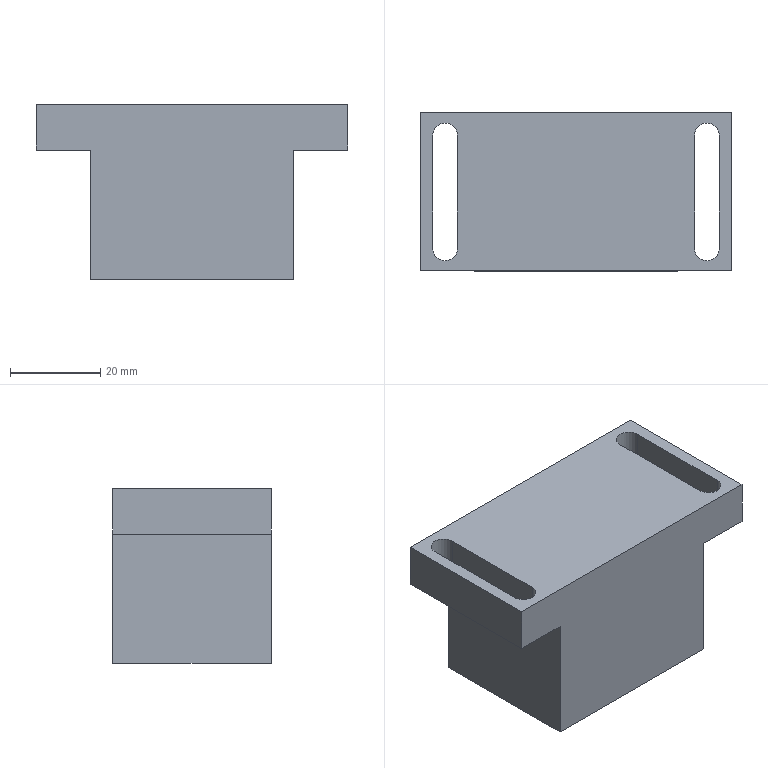Part | STEP file | 11-FG-S00711 | 1 solid | 34 faces | box 69 x 35 x 38.6 mm | volume 65613 mm3 | plane 14 | cylinder 12 | cone 8 | commonest cylinder face diameters 3.3 x8 5.5 x4
STEP:
#1=CARTESIAN_POINT('',(44.15,-7.,10.1));
#2=VERTEX_POINT('',#1);
#3=CARTESIAN_POINT('',(40.85,-7.,10.1));
#4=VERTEX_POINT('',#3);
#5=CARTESIAN_POINT('',(42.5,-7.,10.1));
#6=DIRECTION('',(0.,0.,-1.));
#7=DIRECTION('',(-1.,0.,0.));
#8=AXIS2_PLACEMENT_3D('',#5,#6,#7);
#9=CIRCLE('',#8,1.65);
#10=EDGE_CURVE('',#2,#4,#9,.T.);
#11=ORIENTED_EDGE('',*,*,#10,.F.);
#12=CARTESIAN_POINT('',(44.15,-7.,0.));
#13=VERTEX_POINT('',#12);
#14=CARTESIAN_POINT('',(44.15,-7.,0.));
#15=DIRECTION('',(0.,0.,-1.));
#16=VECTOR('',#15,1000.);
#17=LINE('',#14,#16);
#18=EDGE_CURVE('',#2,#13,#17,.T.);
#19=ORIENTED_EDGE('',*,*,#18,.T.);
#20=CARTESIAN_POINT('',(40.85,-7.,0.));
#21=VERTEX_POINT('',#20);
#22=CARTESIAN_POINT('',(42.5,-7.,0.));
#23=DIRECTION('',(0.,0.,-1.));
#24=DIRECTION('',(-1.,0.,0.));
#25=AXIS2_PLACEMENT_3D('',#22,#23,#24);
#26=CIRCLE('',#25,1.65);
#27=EDGE_CURVE('',#13,#21,#26,.T.);
#28=ORIENTED_EDGE('',*,*,#27,.T.);
#29=CARTESIAN_POINT('',(40.85,-7.,0.));
#30=DIRECTION('',(0.,0.,-1.));
#31=VECTOR('',#30,1000.);
#32=LINE('',#29,#31);
#33=EDGE_CURVE('',#4,#21,#32,.T.);
#34=ORIENTED_EDGE('',*,*,#33,.F.);
#35=EDGE_LOOP('',(#11,#19,#28,#34));
#36=FACE_OUTER_BOUND('',#35,.T.);
#37=CARTESIAN_POINT('',(42.5,-7.,0.));
#38=DIRECTION('',(0.,0.,-1.));
#39=DIRECTION('',(-1.,0.,0.));
#40=AXIS2_PLACEMENT_3D('',#37,#38,#39);
#41=CYLINDRICAL_SURFACE('',#40,1.65);
#42=ADVANCED_FACE('',(#36),#41,.F.);
#43=CARTESIAN_POINT('',(42.5,-7.,11.091));
#44=VERTEX_POINT('',#43);
#45=CARTESIAN_POINT('',(40.85,-7.,10.1));
#46=DIRECTION('',(-0.8572,0.,-0.515));
#47=VECTOR('',#46,1000.);
#48=LINE('',#45,#47);
#49=EDGE_CURVE('',#44,#4,#48,.T.);
#50=ORIENTED_EDGE('',*,*,#49,.F.);
#51=CARTESIAN_POINT('',(44.15,-7.,10.1));
#52=DIRECTION('',(0.8572,0.,-0.515));
#53=VECTOR('',#52,1000.);
#54=LINE('',#51,#53);
#55=EDGE_CURVE('',#44,#2,#54,.T.);
#56=ORIENTED_EDGE('',*,*,#55,.T.);
#57=ORIENTED_EDGE('',*,*,#10,.T.);
#58=EDGE_LOOP('',(#50,#56,#57));
#59=FACE_OUTER_BOUND('',#58,.T.);
#60=CARTESIAN_POINT('',(42.5,-7.,10.1));
#61=DIRECTION('',(0.,0.,-1.));
#62=DIRECTION('',(-1.,0.,0.));
#63=AXIS2_PLACEMENT_3D('',#60,#61,#62);
#64=CONICAL_SURFACE('',#63,1.65,1.03);
#65=ADVANCED_FACE('',(#59),#64,.F.);
#66=CARTESIAN_POINT('',(44.15,-28.,10.1));
#67=VERTEX_POINT('',#66);
#68=CARTESIAN_POINT('',(40.85,-28.,10.1));
#69=VERTEX_POINT('',#68);
#70=CARTESIAN_POINT('',(42.5,-28.,10.1));
#71=DIRECTION('',(0.,0.,-1.));
#72=DIRECTION('',(-1.,0.,0.));
#73=AXIS2_PLACEMENT_3D('',#70,#71,#72);
#74=CIRCLE('',#73,1.65);
#75=EDGE_CURVE('',#67,#69,#74,.T.);
#76=ORIENTED_EDGE('',*,*,#75,.F.);
#77=CARTESIAN_POINT('',(44.15,-28.,0.));
#78=VERTEX_POINT('',#77);
#79=CARTESIAN_POINT('',(44.15,-28.,0.));
#80=DIRECTION('',(0.,0.,-1.));
#81=VECTOR('',#80,1000.);
#82=LINE('',#79,#81);
#83=EDGE_CURVE('',#67,#78,#82,.T.);
#84=ORIENTED_EDGE('',*,*,#83,.T.);
#85=CARTESIAN_POINT('',(40.85,-28.,0.));
#86=VERTEX_POINT('',#85);
#87=CARTESIAN_POINT('',(42.5,-28.,0.));
#88=DIRECTION('',(0.,0.,-1.));
#89=DIRECTION('',(-1.,0.,0.));
#90=AXIS2_PLACEMENT_3D('',#87,#88,#89);
#91=CIRCLE('',#90,1.65);
#92=EDGE_CURVE('',#78,#86,#91,.T.);
#93=ORIENTED_EDGE('',*,*,#92,.T.);
#94=CARTESIAN_POINT('',(40.85,-28.,0.));
#95=DIRECTION('',(0.,0.,-1.));
#96=VECTOR('',#95,1000.);
#97=LINE('',#94,#96);
#98=EDGE_CURVE('',#69,#86,#97,.T.);
#99=ORIENTED_EDGE('',*,*,#98,.F.);
#100=EDGE_LOOP('',(#76,#84,#93,#99));
#101=FACE_OUTER_BOUND('',#100,.T.);
#102=CARTESIAN_POINT('',(42.5,-28.,0.));
#103=DIRECTION('',(0.,0.,-1.));
#104=DIRECTION('',(-1.,0.,0.));
#105=AXIS2_PLACEMENT_3D('',#102,#103,#104);
#106=CYLINDRICAL_SURFACE('',#105,1.65);
#107=ADVANCED_FACE('',(#101),#106,.F.);
#108=CARTESIAN_POINT('',(42.5,-28.,11.091));
#109=VERTEX_POINT('',#108);
#110=CARTESIAN_POINT('',(40.85,-28.,10.1));
#111=DIRECTION('',(-0.8572,0.,-0.515));
#112=VECTOR('',#111,1000.);
#113=LINE('',#110,#112);
#114=EDGE_CURVE('',#109,#69,#113,.T.);
#115=ORIENTED_EDGE('',*,*,#114,.F.);
#116=CARTESIAN_POINT('',(44.15,-28.,10.1));
#117=DIRECTION('',(0.8572,0.,-0.515));
#118=VECTOR('',#117,1000.);
#119=LINE('',#116,#118);
#120=EDGE_CURVE('',#109,#67,#119,.T.);
#121=ORIENTED_EDGE('',*,*,#120,.T.);
#122=ORIENTED_EDGE('',*,*,#75,.T.);
#123=EDGE_LOOP('',(#115,#121,#122));
#124=FACE_OUTER_BOUND('',#123,.T.);
#125=CARTESIAN_POINT('',(42.5,-28.,10.1));
#126=DIRECTION('',(0.,0.,-1.));
#127=DIRECTION('',(-1.,0.,0.));
#128=AXIS2_PLACEMENT_3D('',#125,#126,#127);
#129=CONICAL_SURFACE('',#128,1.65,1.03);
#130=ADVANCED_FACE('',(#124),#129,.F.);
#131=CARTESIAN_POINT('',(6.15,-28.,10.1));
#132=VERTEX_POINT('',#131);
#133=CARTESIAN_POINT('',(2.85,-28.,10.1));
#134=VERTEX_POINT('',#133);
#135=CARTESIAN_POINT('',(4.5,-28.,10.1));
#136=DIRECTION('',(0.,0.,-1.));
#137=DIRECTION('',(-1.,0.,0.));
#138=AXIS2_PLACEMENT_3D('',#135,#136,#137);
#139=CIRCLE('',#138,1.65);
#140=EDGE_CURVE('',#132,#134,#139,.T.);
#141=ORIENTED_EDGE('',*,*,#140,.F.);
#142=CARTESIAN_POINT('',(6.15,-28.,0.));
#143=VERTEX_POINT('',#142);
#144=CARTESIAN_POINT('',(6.15,-28.,0.));
#145=DIRECTION('',(0.,0.,-1.));
#146=VECTOR('',#145,1000.);
#147=LINE('',#144,#146);
#148=EDGE_CURVE('',#132,#143,#147,.T.);
#149=ORIENTED_EDGE('',*,*,#148,.T.);
#150=CARTESIAN_POINT('',(2.85,-28.,0.));
#151=VERTEX_POINT('',#150);
#152=CARTESIAN_POINT('',(4.5,-28.,0.));
#153=DIRECTION('',(0.,0.,-1.));
#154=DIRECTION('',(-1.,0.,0.));
#155=AXIS2_PLACEMENT_3D('',#152,#153,#154);
#156=CIRCLE('',#155,1.65);
#157=EDGE_CURVE('',#143,#151,#156,.T.);
#158=ORIENTED_EDGE('',*,*,#157,.T.);
#159=CARTESIAN_POINT('',(2.85,-28.,0.));
#160=DIRECTION('',(0.,0.,-1.));
#161=VECTOR('',#160,1000.);
#162=LINE('',#159,#161);
#163=EDGE_CURVE('',#134,#151,#162,.T.);
#164=ORIENTED_EDGE('',*,*,#163,.F.);
#165=EDGE_LOOP('',(#141,#149,#158,#164));
#166=FACE_OUTER_BOUND('',#165,.T.);
#167=CARTESIAN_POINT('',(4.5,-28.,0.));
#168=DIRECTION('',(0.,0.,-1.));
#169=DIRECTION('',(-1.,0.,0.));
#170=AXIS2_PLACEMENT_3D('',#167,#168,#169);
#171=CYLINDRICAL_SURFACE('',#170,1.65);
#172=ADVANCED_FACE('',(#166),#171,.F.);
#173=CARTESIAN_POINT('',(4.5,-28.,11.091));
#174=VERTEX_POINT('',#173);
#175=CARTESIAN_POINT('',(2.85,-28.,10.1));
#176=DIRECTION('',(-0.8572,0.,-0.515));
#177=VECTOR('',#176,1000.);
#178=LINE('',#175,#177);
#179=EDGE_CURVE('',#174,#134,#178,.T.);
#180=ORIENTED_EDGE('',*,*,#179,.F.);
#181=CARTESIAN_POINT('',(6.15,-28.,10.1));
#182=DIRECTION('',(0.8572,0.,-0.515));
#183=VECTOR('',#182,1000.);
#184=LINE('',#181,#183);
#185=EDGE_CURVE('',#174,#132,#184,.T.);
#186=ORIENTED_EDGE('',*,*,#185,.T.);
#187=ORIENTED_EDGE('',*,*,#140,.T.);
#188=EDGE_LOOP('',(#180,#186,#187));
#189=FACE_OUTER_BOUND('',#188,.T.);
#190=CARTESIAN_POINT('',(4.5,-28.,10.1));
#191=DIRECTION('',(0.,0.,-1.));
#192=DIRECTION('',(-1.,0.,0.));
#193=AXIS2_PLACEMENT_3D('',#190,#191,#192);
#194=CONICAL_SURFACE('',#193,1.65,1.03);
#195=ADVANCED_FACE('',(#189),#194,.F.);
#196=CARTESIAN_POINT('',(6.15,-7.,10.1));
#197=VERTEX_POINT('',#196);
#198=CARTESIAN_POINT('',(2.85,-7.,10.1));
#199=VERTEX_POINT('',#198);
#200=CARTESIAN_POINT('',(4.5,-7.,10.1));
#201=DIRECTION('',(0.,0.,-1.));
#202=DIRECTION('',(-1.,0.,0.));
#203=AXIS2_PLACEMENT_3D('',#200,#201,#202);
#204=CIRCLE('',#203,1.65);
#205=EDGE_CURVE('',#197,#199,#204,.T.);
#206=ORIENTED_EDGE('',*,*,#205,.F.);
#207=CARTESIAN_POINT('',(6.15,-7.,0.));
#208=VERTEX_POINT('',#207);
#209=CARTESIAN_POINT('',(6.15,-7.,0.));
#210=DIRECTION('',(0.,0.,-1.));
#211=VECTOR('',#210,1000.);
#212=LINE('',#209,#211);
#213=EDGE_CURVE('',#197,#208,#212,.T.);
#214=ORIENTED_EDGE('',*,*,#213,.T.);
#215=CARTESIAN_POINT('',(2.85,-7.,0.));
#216=VERTEX_POINT('',#215);
#217=CARTESIAN_POINT('',(4.5,-7.,0.));
#218=DIRECTION('',(0.,0.,-1.));
#219=DIRECTION('',(-1.,0.,0.));
#220=AXIS2_PLACEMENT_3D('',#217,#218,#219);
#221=CIRCLE('',#220,1.65);
#222=EDGE_CURVE('',#208,#216,#221,.T.);
#223=ORIENTED_EDGE('',*,*,#222,.T.);
#224=CARTESIAN_POINT('',(2.85,-7.,0.));
#225=DIRECTION('',(0.,0.,-1.));
#226=VECTOR('',#225,1000.);
#227=LINE('',#224,#226);
#228=EDGE_CURVE('',#199,#216,#227,.T.);
#229=ORIENTED_EDGE('',*,*,#228,.F.);
#230=EDGE_LOOP('',(#206,#214,#223,#229));
#231=FACE_OUTER_BOUND('',#230,.T.);
#232=CARTESIAN_POINT('',(4.5,-7.,0.));
#233=DIRECTION('',(0.,0.,-1.));
#234=DIRECTION('',(-1.,0.,0.));
#235=AXIS2_PLACEMENT_3D('',#232,#233,#234);
#236=CYLINDRICAL_SURFACE('',#235,1.65);
#237=ADVANCED_FACE('',(#231),#236,.F.);
#238=CARTESIAN_POINT('',(4.5,-7.,11.091));
#239=VERTEX_POINT('',#238);
#240=CARTESIAN_POINT('',(2.85,-7.,10.1));
#241=DIRECTION('',(-0.8572,0.,-0.515));
#242=VECTOR('',#241,1000.);
#243=LINE('',#240,#242);
#244=EDGE_CURVE('',#239,#199,#243,.T.);
#245=ORIENTED_EDGE('',*,*,#244,.F.);
#246=CARTESIAN_POINT('',(6.15,-7.,10.1));
#247=DIRECTION('',(0.8572,0.,-0.515));
#248=VECTOR('',#247,1000.);
#249=LINE('',#246,#248);
#250=EDGE_CURVE('',#239,#197,#249,.T.);
#251=ORIENTED_EDGE('',*,*,#250,.T.);
#252=ORIENTED_EDGE('',*,*,#205,.T.);
#253=EDGE_LOOP('',(#245,#251,#252));
#254=FACE_OUTER_BOUND('',#253,.T.);
#255=CARTESIAN_POINT('',(4.5,-7.,10.1));
#256=DIRECTION('',(0.,0.,-1.));
#257=DIRECTION('',(-1.,0.,0.));
#258=AXIS2_PLACEMENT_3D('',#255,#256,#257);
#259=CONICAL_SURFACE('',#258,1.65,1.03);
#260=ADVANCED_FACE('',(#254),#259,.F.);
#261=CARTESIAN_POINT('',(-11.,-35.,38.6));
#262=VERTEX_POINT('',#261);
#263=CARTESIAN_POINT('',(58.,-35.,38.6));
#264=VERTEX_POINT('',#263);
#265=CARTESIAN_POINT('',(0.,-35.,38.6));
#266=DIRECTION('',(1.,0.,0.));
#267=VECTOR('',#266,1000.);
#268=LINE('',#265,#267);
#269=EDGE_CURVE('',#262,#264,#268,.T.);
#270=ORIENTED_EDGE('',*,*,#269,.F.);
#271=CARTESIAN_POINT('',(-11.,-35.,28.6));
#272=VERTEX_POINT('',#271);
#273=CARTESIAN_POINT('',(-11.,-35.,28.6));
#274=DIRECTION('',(0.,0.,1.));
#275=VECTOR('',#274,1000.);
#276=LINE('',#273,#275);
#277=EDGE_CURVE('',#272,#262,#276,.T.);
#278=ORIENTED_EDGE('',*,*,#277,.F.);
#279=CARTESIAN_POINT('',(1.,-35.,28.6));
#280=VERTEX_POINT('',#279);
#281=CARTESIAN_POINT('',(1.,-35.,28.6));
#282=DIRECTION('',(1.,0.,0.));
#283=VECTOR('',#282,1000.);
#284=LINE('',#281,#283);
#285=EDGE_CURVE('',#272,#280,#284,.T.);
#286=ORIENTED_EDGE('',*,*,#285,.T.);
#287=CARTESIAN_POINT('',(1.,-35.,0.));
#288=VERTEX_POINT('',#287);
#289=CARTESIAN_POINT('',(1.,-35.,38.6));
#290=DIRECTION('',(0.,0.,-1.));
#291=VECTOR('',#290,1000.);
#292=LINE('',#289,#291);
#293=EDGE_CURVE('',#280,#288,#292,.T.);
#294=ORIENTED_EDGE('',*,*,#293,.T.);
#295=CARTESIAN_POINT('',(46.,-35.,0.));
#296=VERTEX_POINT('',#295);
#297=CARTESIAN_POINT('',(0.,-35.,0.));
#298=DIRECTION('',(1.,0.,0.));
#299=VECTOR('',#298,1000.);
#300=LINE('',#297,#299);
#301=EDGE_CURVE('',#288,#296,#300,.T.);
#302=ORIENTED_EDGE('',*,*,#301,.T.);
#303=CARTESIAN_POINT('',(46.,-35.,28.6));
#304=VERTEX_POINT('',#303);
#305=CARTESIAN_POINT('',(46.,-35.,38.6));
#306=DIRECTION('',(0.,0.,-1.));
#307=VECTOR('',#306,1000.);
#308=LINE('',#305,#307);
#309=EDGE_CURVE('',#304,#296,#308,.T.);
#310=ORIENTED_EDGE('',*,*,#309,.F.);
#311=CARTESIAN_POINT('',(58.,-35.,28.6));
#312=VERTEX_POINT('',#311);
#313=CARTESIAN_POINT('',(46.,-35.,28.6));
#314=DIRECTION('',(1.,0.,0.));
#315=VECTOR('',#314,1000.);
#316=LINE('',#313,#315);
#317=EDGE_CURVE('',#304,#312,#316,.T.);
#318=ORIENTED_EDGE('',*,*,#317,.T.);
#319=CARTESIAN_POINT('',(58.,-35.,28.6));
#320=DIRECTION('',(0.,0.,1.));
#321=VECTOR('',#320,1000.);
#322=LINE('',#319,#321);
#323=EDGE_CURVE('',#312,#264,#322,.T.);
#324=ORIENTED_EDGE('',*,*,#323,.T.);
#325=EDGE_LOOP('',(#270,#278,#286,#294,#302,#310,#318,#324));
#326=FACE_OUTER_BOUND('',#325,.T.);
#327=CARTESIAN_POINT('',(0.,-35.,38.6));
#328=DIRECTION('',(0.,1.,0.));
#329=DIRECTION('',(0.,0.,1.));
#330=AXIS2_PLACEMENT_3D('',#327,#328,#329);
#331=PLANE('',#330);
#332=ADVANCED_FACE('',(#326),#331,.F.);
#333=CARTESIAN_POINT('',(46.,0.,28.6));
#334=VERTEX_POINT('',#333);
#335=CARTESIAN_POINT('',(46.,0.,0.));
#336=VERTEX_POINT('',#335);
#337=CARTESIAN_POINT('',(46.,0.,38.6));
#338=DIRECTION('',(0.,0.,-1.));
#339=VECTOR('',#338,1000.);
#340=LINE('',#337,#339);
#341=EDGE_CURVE('',#334,#336,#340,.T.);
#342=ORIENTED_EDGE('',*,*,#341,.F.);
#343=CARTESIAN_POINT('',(46.,0.,28.6));
#344=DIRECTION('',(0.,-1.,0.));
#345=VECTOR('',#344,1000.);
#346=LINE('',#343,#345);
#347=EDGE_CURVE('',#334,#304,#346,.T.);
#348=ORIENTED_EDGE('',*,*,#347,.T.);
#349=ORIENTED_EDGE('',*,*,#309,.T.);
#350=CARTESIAN_POINT('',(46.,0.,0.));
#351=DIRECTION('',(0.,1.,0.));
#352=VECTOR('',#351,1000.);
#353=LINE('',#350,#352);
#354=EDGE_CURVE('',#296,#336,#353,.T.);
#355=ORIENTED_EDGE('',*,*,#354,.T.);
#356=EDGE_LOOP('',(#342,#348,#349,#355));
#357=FACE_OUTER_BOUND('',#356,.T.);
#358=CARTESIAN_POINT('',(46.,0.,38.6));
#359=DIRECTION('',(-1.,0.,0.));
#360=DIRECTION('',(0.,0.,1.));
#361=AXIS2_PLACEMENT_3D('',#358,#359,#360);
#362=PLANE('',#361);
#363=ADVANCED_FACE('',(#357),#362,.F.);
#364=CARTESIAN_POINT('',(1.,0.,0.));
#365=VERTEX_POINT('',#364);
#366=CARTESIAN_POINT('',(0.,0.,0.));
#367=DIRECTION('',(-1.,0.,0.));
#368=VECTOR('',#367,1000.);
#369=LINE('',#366,#368);
#370=EDGE_CURVE('',#336,#365,#369,.T.);
#371=ORIENTED_EDGE('',*,*,#370,.T.);
#372=CARTESIAN_POINT('',(1.,0.,28.6));
#373=VERTEX_POINT('',#372);
#374=CARTESIAN_POINT('',(1.,0.,0.));
#375=DIRECTION('',(0.,0.,-1.));
#376=VECTOR('',#375,1000.);
#377=LINE('',#374,#376);
#378=EDGE_CURVE('',#373,#365,#377,.T.);
#379=ORIENTED_EDGE('',*,*,#378,.F.);
#380=CARTESIAN_POINT('',(-11.,0.,28.6));
#381=VERTEX_POINT('',#380);
#382=CARTESIAN_POINT('',(1.,0.,28.6));
#383=DIRECTION('',(-1.,0.,0.));
#384=VECTOR('',#383,1000.);
#385=LINE('',#382,#384);
#386=EDGE_CURVE('',#373,#381,#385,.T.);
#387=ORIENTED_EDGE('',*,*,#386,.T.);
#388=CARTESIAN_POINT('',(-11.,0.,38.6));
#389=VERTEX_POINT('',#388);
#390=CARTESIAN_POINT('',(-11.,0.,28.6));
#391=DIRECTION('',(0.,0.,1.));
#392=VECTOR('',#391,1000.);
#393=LINE('',#390,#392);
#394=EDGE_CURVE('',#381,#389,#393,.T.);
#395=ORIENTED_EDGE('',*,*,#394,.T.);
#396=CARTESIAN_POINT('',(58.,0.,38.6));
#397=VERTEX_POINT('',#396);
#398=CARTESIAN_POINT('',(0.,0.,38.6));
#399=DIRECTION('',(-1.,0.,0.));
#400=VECTOR('',#399,1000.);
#401=LINE('',#398,#400);
#402=EDGE_CURVE('',#397,#389,#401,.T.);
#403=ORIENTED_EDGE('',*,*,#402,.F.);
#404=CARTESIAN_POINT('',(58.,0.,28.6));
#405=VERTEX_POINT('',#404);
#406=CARTESIAN_POINT('',(58.,0.,28.6));
#407=DIRECTION('',(0.,0.,1.));
#408=VECTOR('',#407,1000.);
#409=LINE('',#406,#408);
#410=EDGE_CURVE('',#405,#397,#409,.T.);
#411=ORIENTED_EDGE('',*,*,#410,.F.);
#412=CARTESIAN_POINT('',(46.,0.,28.6));
#413=DIRECTION('',(-1.,0.,0.));
#414=VECTOR('',#413,1000.);
#415=LINE('',#412,#414);
#416=EDGE_CURVE('',#405,#334,#415,.T.);
#417=ORIENTED_EDGE('',*,*,#416,.T.);
#418=ORIENTED_EDGE('',*,*,#341,.T.);
#419=EDGE_LOOP('',(#371,#379,#387,#395,#403,#411,#417,#418));
#420=FACE_OUTER_BOUND('',#419,.T.);
#421=CARTESIAN_POINT('',(0.,0.,38.6));
#422=DIRECTION('',(0.,-1.,0.));
#423=DIRECTION('',(0.,0.,-1.));
#424=AXIS2_PLACEMENT_3D('',#421,#422,#423);
#425=PLANE('',#424);
#426=ADVANCED_FACE('',(#420),#425,.F.);
#427=CARTESIAN_POINT('',(-2.75,-5.,38.6));
#428=VERTEX_POINT('',#427);
#429=CARTESIAN_POINT('',(-8.25,-5.,38.6));
#430=VERTEX_POINT('',#429);
#431=CARTESIAN_POINT('',(-5.5,-5.,38.6));
#432=DIRECTION('',(0.,0.,1.));
#433=DIRECTION('',(1.,0.,0.));
#434=AXIS2_PLACEMENT_3D('',#431,#432,#433);
#435=CIRCLE('',#434,2.75);
#436=EDGE_CURVE('',#428,#430,#435,.T.);
#437=ORIENTED_EDGE('',*,*,#436,.F.);
#438=CARTESIAN_POINT('',(-2.75,-30.,38.6));
#439=VERTEX_POINT('',#438);
#440=CARTESIAN_POINT('',(-2.75,0.,38.6));
#441=DIRECTION('',(0.,1.,0.));
#442=VECTOR('',#441,1000.);
#443=LINE('',#440,#442);
#444=EDGE_CURVE('',#439,#428,#443,.T.);
#445=ORIENTED_EDGE('',*,*,#444,.F.);
#446=CARTESIAN_POINT('',(-8.25,-30.,38.6));
#447=VERTEX_POINT('',#446);
#448=CARTESIAN_POINT('',(-5.5,-30.,38.6));
#449=DIRECTION('',(0.,0.,1.));
#450=DIRECTION('',(1.,0.,0.));
#451=AXIS2_PLACEMENT_3D('',#448,#449,#450);
#452=CIRCLE('',#451,2.75);
#453=EDGE_CURVE('',#447,#439,#452,.T.);
#454=ORIENTED_EDGE('',*,*,#453,.F.);
#455=CARTESIAN_POINT('',(-8.25,0.,38.6));
#456=DIRECTION('',(0.,-1.,0.));
#457=VECTOR('',#456,1000.);
#458=LINE('',#455,#457);
#459=EDGE_CURVE('',#430,#447,#458,.T.);
#460=ORIENTED_EDGE('',*,*,#459,.F.);
#461=EDGE_LOOP('',(#437,#445,#454,#460));
#462=FACE_BOUND('',#461,.T.);
#463=CARTESIAN_POINT('',(55.25,-5.,38.6));
#464=VERTEX_POINT('',#463);
#465=CARTESIAN_POINT('',(49.75,-5.,38.6));
#466=VERTEX_POINT('',#465);
#467=CARTESIAN_POINT('',(52.5,-5.,38.6));
#468=DIRECTION('',(0.,0.,1.));
#469=DIRECTION('',(1.,0.,0.));
#470=AXIS2_PLACEMENT_3D('',#467,#468,#469);
#471=CIRCLE('',#470,2.75);
#472=EDGE_CURVE('',#464,#466,#471,.T.);
#473=ORIENTED_EDGE('',*,*,#472,.F.);
#474=CARTESIAN_POINT('',(55.25,-30.,38.6));
#475=VERTEX_POINT('',#474);
#476=CARTESIAN_POINT('',(55.25,0.,38.6));
#477=DIRECTION('',(0.,1.,0.));
#478=VECTOR('',#477,1000.);
#479=LINE('',#476,#478);
#480=EDGE_CURVE('',#475,#464,#479,.T.);
#481=ORIENTED_EDGE('',*,*,#480,.F.);
#482=CARTESIAN_POINT('',(49.75,-30.,38.6));
#483=VERTEX_POINT('',#482);
#484=CARTESIAN_POINT('',(52.5,-30.,38.6));
#485=DIRECTION('',(0.,0.,1.));
#486=DIRECTION('',(1.,0.,0.));
#487=AXIS2_PLACEMENT_3D('',#484,#485,#486);
#488=CIRCLE('',#487,2.75);
#489=EDGE_CURVE('',#483,#475,#488,.T.);
#490=ORIENTED_EDGE('',*,*,#489,.F.);
#491=CARTESIAN_POINT('',(49.75,0.,38.6));
#492=DIRECTION('',(0.,-1.,0.));
#493=VECTOR('',#492,1000.);
#494=LINE('',#491,#493);
#495=EDGE_CURVE('',#466,#483,#494,.T.);
#496=ORIENTED_EDGE('',*,*,#495,.F.);
#497=EDGE_LOOP('',(#473,#481,#490,#496));
#498=FACE_BOUND('',#497,.T.);
#499=ORIENTED_EDGE('',*,*,#402,.T.);
#500=CARTESIAN_POINT('',(-11.,0.,38.6));
#501=DIRECTION('',(0.,-1.,0.));
#502=VECTOR('',#501,1000.);
#503=LINE('',#500,#502);
#504=EDGE_CURVE('',#389,#262,#503,.T.);
#505=ORIENTED_EDGE('',*,*,#504,.T.);
#506=ORIENTED_EDGE('',*,*,#269,.T.);
#507=CARTESIAN_POINT('',(58.,0.,38.6));
#508=DIRECTION('',(0.,1.,0.));
#509=VECTOR('',#508,1000.);
#510=LINE('',#507,#509);
#511=EDGE_CURVE('',#264,#397,#510,.T.);
#512=ORIENTED_EDGE('',*,*,#511,.T.);
#513=EDGE_LOOP('',(#499,#505,#506,#512));
#514=FACE_OUTER_BOUND('',#513,.T.);
#515=CARTESIAN_POINT('',(0.,0.,38.6));
#516=DIRECTION('',(0.,0.,1.));
#517=DIRECTION('',(1.,0.,0.));
#518=AXIS2_PLACEMENT_3D('',#515,#516,#517);
#519=PLANE('',#518);
#520=ADVANCED_FACE('',(#462,#498,#514),#519,.T.);
#521=CARTESIAN_POINT('',(42.5,-7.,0.));
#522=DIRECTION('',(0.,0.,-1.));
#523=DIRECTION('',(-1.,0.,0.));
#524=AXIS2_PLACEMENT_3D('',#521,#522,#523);
#525=CIRCLE('',#524,1.65);
#526=EDGE_CURVE('',#21,#13,#525,.T.);
#527=ORIENTED_EDGE('',*,*,#526,.F.);
#528=ORIENTED_EDGE('',*,*,#27,.F.);
#529=EDGE_LOOP('',(#527,#528));
#530=FACE_BOUND('',#529,.T.);
#531=CARTESIAN_POINT('',(42.5,-28.,0.));
#532=DIRECTION('',(0.,0.,-1.));
#533=DIRECTION('',(-1.,0.,0.));
#534=AXIS2_PLACEMENT_3D('',#531,#532,#533);
#535=CIRCLE('',#534,1.65);
#536=EDGE_CURVE('',#86,#78,#535,.T.);
#537=ORIENTED_EDGE('',*,*,#536,.F.);
#538=ORIENTED_EDGE('',*,*,#92,.F.);
#539=EDGE_LOOP('',(#537,#538));
#540=FACE_BOUND('',#539,.T.);
#541=CARTESIAN_POINT('',(4.5,-28.,0.));
#542=DIRECTION('',(0.,0.,-1.));
#543=DIRECTION('',(-1.,0.,0.));
#544=AXIS2_PLACEMENT_3D('',#541,#542,#543);
#545=CIRCLE('',#544,1.65);
#546=EDGE_CURVE('',#151,#143,#545,.T.);
#547=ORIENTED_EDGE('',*,*,#546,.F.);
#548=ORIENTED_EDGE('',*,*,#157,.F.);
#549=EDGE_LOOP('',(#547,#548));
#550=FACE_BOUND('',#549,.T.);
#551=CARTESIAN_POINT('',(4.5,-7.,0.));
#552=DIRECTION('',(0.,0.,-1.));
#553=DIRECTION('',(-1.,0.,0.));
#554=AXIS2_PLACEMENT_3D('',#551,#552,#553);
#555=CIRCLE('',#554,1.65);
#556=EDGE_CURVE('',#216,#208,#555,.T.);
#557=ORIENTED_EDGE('',*,*,#556,.F.);
#558=ORIENTED_EDGE('',*,*,#222,.F.);
#559=EDGE_LOOP('',(#557,#558));
#560=FACE_BOUND('',#559,.T.);
#561=ORIENTED_EDGE('',*,*,#301,.F.);
#562=CARTESIAN_POINT('',(1.,0.,0.));
#563=DIRECTION('',(0.,1.,0.));
#564=VECTOR('',#563,1000.);
#565=LINE('',#562,#564);
#566=EDGE_CURVE('',#288,#365,#565,.T.);
#567=ORIENTED_EDGE('',*,*,#566,.T.);
#568=ORIENTED_EDGE('',*,*,#370,.F.);
#569=ORIENTED_EDGE('',*,*,#354,.F.);
#570=EDGE_LOOP('',(#561,#567,#568,#569));
#571=FACE_OUTER_BOUND('',#570,.T.);
#572=CARTESIAN_POINT('',(0.,0.,0.));
#573=DIRECTION('',(0.,0.,1.));
#574=DIRECTION('',(1.,0.,0.));
#575=AXIS2_PLACEMENT_3D('',#572,#573,#574);
#576=PLANE('',#575);
#577=ADVANCED_FACE('',(#530,#540,#550,#560,#571),#576,.F.);
#578=ORIENTED_EDGE('',*,*,#293,.F.);
#579=CARTESIAN_POINT('',(1.,0.,28.6));
#580=DIRECTION('',(0.,1.,0.));
#581=VECTOR('',#580,1000.);
#582=LINE('',#579,#581);
#583=EDGE_CURVE('',#280,#373,#582,.T.);
#584=ORIENTED_EDGE('',*,*,#583,.T.);
#585=ORIENTED_EDGE('',*,*,#378,.T.);
#586=ORIENTED_EDGE('',*,*,#566,.F.);
#587=EDGE_LOOP('',(#578,#584,#585,#586));
#588=FACE_OUTER_BOUND('',#587,.T.);
#589=CARTESIAN_POINT('',(1.,-42.,0.));
#590=DIRECTION('',(1.,0.,0.));
#591=DIRECTION('',(0.,0.,-1.));
#592=AXIS2_PLACEMENT_3D('',#589,#590,#591);
#593=PLANE('',#592);
#594=ADVANCED_FACE('',(#588),#593,.F.);
#595=ORIENTED_EDGE('',*,*,#250,.F.);
#596=ORIENTED_EDGE('',*,*,#244,.T.);
#597=CARTESIAN_POINT('',(4.5,-7.,10.1));
#598=DIRECTION('',(0.,0.,-1.));
#599=DIRECTION('',(-1.,0.,0.));
#600=AXIS2_PLACEMENT_3D('',#597,#598,#599);
#601=CIRCLE('',#600,1.65);
#602=EDGE_CURVE('',#199,#197,#601,.T.);
#603=ORIENTED_EDGE('',*,*,#602,.T.);
#604=EDGE_LOOP('',(#595,#596,#603));
#605=FACE_OUTER_BOUND('',#604,.T.);
#606=CARTESIAN_POINT('',(4.5,-7.,10.1));
#607=DIRECTION('',(0.,0.,-1.));
#608=DIRECTION('',(-1.,0.,0.));
#609=AXIS2_PLACEMENT_3D('',#606,#607,#608);
#610=CONICAL_SURFACE('',#609,1.65,1.03);
#611=ADVANCED_FACE('',(#605),#610,.F.);
#612=ORIENTED_EDGE('',*,*,#213,.F.);
#613=ORIENTED_EDGE('',*,*,#602,.F.);
#614=ORIENTED_EDGE('',*,*,#228,.T.);
#615=ORIENTED_EDGE('',*,*,#556,.T.);
#616=EDGE_LOOP('',(#612,#613,#614,#615));
#617=FACE_OUTER_BOUND('',#616,.T.);
#618=CARTESIAN_POINT('',(4.5,-7.,0.));
#619=DIRECTION('',(0.,0.,-1.));
#620=DIRECTION('',(-1.,0.,0.));
#621=AXIS2_PLACEMENT_3D('',#618,#619,#620);
#622=CYLINDRICAL_SURFACE('',#621,1.65);
#623=ADVANCED_FACE('',(#617),#622,.F.);
#624=ORIENTED_EDGE('',*,*,#185,.F.);
#625=ORIENTED_EDGE('',*,*,#179,.T.);
#626=CARTESIAN_POINT('',(4.5,-28.,10.1));
#627=DIRECTION('',(0.,0.,-1.));
#628=DIRECTION('',(-1.,0.,0.));
#629=AXIS2_PLACEMENT_3D('',#626,#627,#628);
#630=CIRCLE('',#629,1.65);
#631=EDGE_CURVE('',#134,#132,#630,.T.);
#632=ORIENTED_EDGE('',*,*,#631,.T.);
#633=EDGE_LOOP('',(#624,#625,#632));
#634=FACE_OUTER_BOUND('',#633,.T.);
#635=CARTESIAN_POINT('',(4.5,-28.,10.1));
#636=DIRECTION('',(0.,0.,-1.));
#637=DIRECTION('',(-1.,0.,0.));
#638=AXIS2_PLACEMENT_3D('',#635,#636,#637);
#639=CONICAL_SURFACE('',#638,1.65,1.03);
#640=ADVANCED_FACE('',(#634),#639,.F.);
#641=ORIENTED_EDGE('',*,*,#148,.F.);
#642=ORIENTED_EDGE('',*,*,#631,.F.);
#643=ORIENTED_EDGE('',*,*,#163,.T.);
#644=ORIENTED_EDGE('',*,*,#546,.T.);
#645=EDGE_LOOP('',(#641,#642,#643,#644));
#646=FACE_OUTER_BOUND('',#645,.T.);
#647=CARTESIAN_POINT('',(4.5,-28.,0.));
#648=DIRECTION('',(0.,0.,-1.));
#649=DIRECTION('',(-1.,0.,0.));
#650=AXIS2_PLACEMENT_3D('',#647,#648,#649);
#651=CYLINDRICAL_SURFACE('',#650,1.65);
#652=ADVANCED_FACE('',(#646),#651,.F.);
#653=ORIENTED_EDGE('',*,*,#120,.F.);
#654=ORIENTED_EDGE('',*,*,#114,.T.);
#655=CARTESIAN_POINT('',(42.5,-28.,10.1));
#656=DIRECTION('',(0.,0.,-1.));
#657=DIRECTION('',(-1.,0.,0.));
#658=AXIS2_PLACEMENT_3D('',#655,#656,#657);
#659=CIRCLE('',#658,1.65);
#660=EDGE_CURVE('',#69,#67,#659,.T.);
#661=ORIENTED_EDGE('',*,*,#660,.T.);
#662=EDGE_LOOP('',(#653,#654,#661));
#663=FACE_OUTER_BOUND('',#662,.T.);
#664=CARTESIAN_POINT('',(42.5,-28.,10.1));
#665=DIRECTION('',(0.,0.,-1.));
#666=DIRECTION('',(-1.,0.,0.));
#667=AXIS2_PLACEMENT_3D('',#664,#665,#666);
#668=CONICAL_SURFACE('',#667,1.65,1.03);
#669=ADVANCED_FACE('',(#663),#668,.F.);
#670=ORIENTED_EDGE('',*,*,#83,.F.);
#671=ORIENTED_EDGE('',*,*,#660,.F.);
#672=ORIENTED_EDGE('',*,*,#98,.T.);
#673=ORIENTED_EDGE('',*,*,#536,.T.);
#674=EDGE_LOOP('',(#670,#671,#672,#673));
#675=FACE_OUTER_BOUND('',#674,.T.);
#676=CARTESIAN_POINT('',(42.5,-28.,0.));
#677=DIRECTION('',(0.,0.,-1.));
#678=DIRECTION('',(-1.,0.,0.));
#679=AXIS2_PLACEMENT_3D('',#676,#677,#678);
#680=CYLINDRICAL_SURFACE('',#679,1.65);
#681=ADVANCED_FACE('',(#675),#680,.F.);
#682=ORIENTED_EDGE('',*,*,#55,.F.);
#683=ORIENTED_EDGE('',*,*,#49,.T.);
#684=CARTESIAN_POINT('',(42.5,-7.,10.1));
#685=DIRECTION('',(0.,0.,-1.));
#686=DIRECTION('',(-1.,0.,0.));
#687=AXIS2_PLACEMENT_3D('',#684,#685,#686);
#688=CIRCLE('',#687,1.65);
#689=EDGE_CURVE('',#4,#2,#688,.T.);
#690=ORIENTED_EDGE('',*,*,#689,.T.);
#691=EDGE_LOOP('',(#682,#683,#690));
#692=FACE_OUTER_BOUND('',#691,.T.);
#693=CARTESIAN_POINT('',(42.5,-7.,10.1));
#694=DIRECTION('',(0.,0.,-1.));
#695=DIRECTION('',(-1.,0.,0.));
#696=AXIS2_PLACEMENT_3D('',#693,#694,#695);
#697=CONICAL_SURFACE('',#696,1.65,1.03);
#698=ADVANCED_FACE('',(#692),#697,.F.);
#699=ORIENTED_EDGE('',*,*,#18,.F.);
#700=ORIENTED_EDGE('',*,*,#689,.F.);
#701=ORIENTED_EDGE('',*,*,#33,.T.);
#702=ORIENTED_EDGE('',*,*,#526,.T.);
#703=EDGE_LOOP('',(#699,#700,#701,#702));
#704=FACE_OUTER_BOUND('',#703,.T.);
#705=CARTESIAN_POINT('',(42.5,-7.,0.));
#706=DIRECTION('',(0.,0.,-1.));
#707=DIRECTION('',(-1.,0.,0.));
#708=AXIS2_PLACEMENT_3D('',#705,#706,#707);
#709=CYLINDRICAL_SURFACE('',#708,1.65);
#710=ADVANCED_FACE('',(#704),#709,.F.);
#711=ORIENTED_EDGE('',*,*,#504,.F.);
#712=ORIENTED_EDGE('',*,*,#394,.F.);
#713=CARTESIAN_POINT('',(-11.,0.,28.6));
#714=DIRECTION('',(0.,-1.,0.));
#715=VECTOR('',#714,1000.);
#716=LINE('',#713,#715);
#717=EDGE_CURVE('',#381,#272,#716,.T.);
#718=ORIENTED_EDGE('',*,*,#717,.T.);
#719=ORIENTED_EDGE('',*,*,#277,.T.);
#720=EDGE_LOOP('',(#711,#712,#718,#719));
#721=FACE_OUTER_BOUND('',#720,.T.);
#722=CARTESIAN_POINT('',(-11.,0.,28.6));
#723=DIRECTION('',(-1.,0.,0.));
#724=DIRECTION('',(0.,-1.,0.));
#725=AXIS2_PLACEMENT_3D('',#722,#723,#724);
#726=PLANE('',#725);
#727=ADVANCED_FACE('',(#721),#726,.T.);
#728=CARTESIAN_POINT('',(-8.25,-5.,28.6));
#729=VERTEX_POINT('',#728);
#730=CARTESIAN_POINT('',(-2.75,-5.,28.6));
#731=VERTEX_POINT('',#730);
#732=CARTESIAN_POINT('',(-5.5,-5.,28.6));
#733=DIRECTION('',(0.,0.,-1.));
#734=DIRECTION('',(-1.,0.,0.));
#735=AXIS2_PLACEMENT_3D('',#732,#733,#734);
#736=CIRCLE('',#735,2.75);
#737=EDGE_CURVE('',#729,#731,#736,.T.);
#738=ORIENTED_EDGE('',*,*,#737,.F.);
#739=CARTESIAN_POINT('',(-8.25,-30.,28.6));
#740=VERTEX_POINT('',#739);
#741=CARTESIAN_POINT('',(-8.25,-5.,28.6));
#742=DIRECTION('',(0.,1.,0.));
#743=VECTOR('',#742,1000.);
#744=LINE('',#741,#743);
#745=EDGE_CURVE('',#740,#729,#744,.T.);
#746=ORIENTED_EDGE('',*,*,#745,.F.);
#747=CARTESIAN_POINT('',(-2.75,-30.,28.6));
#748=VERTEX_POINT('',#747);
#749=CARTESIAN_POINT('',(-5.5,-30.,28.6));
#750=DIRECTION('',(0.,0.,-1.));
#751=DIRECTION('',(-1.,0.,0.));
#752=AXIS2_PLACEMENT_3D('',#749,#750,#751);
#753=CIRCLE('',#752,2.75);
#754=EDGE_CURVE('',#748,#740,#753,.T.);
#755=ORIENTED_EDGE('',*,*,#754,.F.);
#756=CARTESIAN_POINT('',(-2.75,-5.,28.6));
#757=DIRECTION('',(0.,-1.,0.));
#758=VECTOR('',#757,1000.);
#759=LINE('',#756,#758);
#760=EDGE_CURVE('',#731,#748,#759,.T.);
#761=ORIENTED_EDGE('',*,*,#760,.F.);
#762=EDGE_LOOP('',(#738,#746,#755,#761));
#763=FACE_BOUND('',#762,.T.);
#764=ORIENTED_EDGE('',*,*,#583,.F.);
#765=ORIENTED_EDGE('',*,*,#285,.F.);
#766=ORIENTED_EDGE('',*,*,#717,.F.);
#767=ORIENTED_EDGE('',*,*,#386,.F.);
#768=EDGE_LOOP('',(#764,#765,#766,#767));
#769=FACE_OUTER_BOUND('',#768,.T.);
#770=CARTESIAN_POINT('',(0.,0.,28.6));
#771=DIRECTION('',(0.,0.,-1.));
#772=DIRECTION('',(-1.,0.,0.));
#773=AXIS2_PLACEMENT_3D('',#770,#771,#772);
#774=PLANE('',#773);
#775=ADVANCED_FACE('',(#763,#769),#774,.T.);
#776=ORIENTED_EDGE('',*,*,#511,.F.);
#777=ORIENTED_EDGE('',*,*,#323,.F.);
#778=CARTESIAN_POINT('',(58.,0.,28.6));
#779=DIRECTION('',(0.,1.,0.));
#780=VECTOR('',#779,1000.);
#781=LINE('',#778,#780);
#782=EDGE_CURVE('',#312,#405,#781,.T.);
#783=ORIENTED_EDGE('',*,*,#782,.T.);
#784=ORIENTED_EDGE('',*,*,#410,.T.);
#785=EDGE_LOOP('',(#776,#777,#783,#784));
#786=FACE_OUTER_BOUND('',#785,.T.);
#787=CARTESIAN_POINT('',(58.,0.,28.6));
#788=DIRECTION('',(1.,0.,0.));
#789=DIRECTION('',(0.,1.,0.));
#790=AXIS2_PLACEMENT_3D('',#787,#788,#789);
#791=PLANE('',#790);
#792=ADVANCED_FACE('',(#786),#791,.T.);
#793=CARTESIAN_POINT('',(55.25,-5.,28.6));
#794=VERTEX_POINT('',#793);
#795=CARTESIAN_POINT('',(55.25,-30.,28.6));
#796=VERTEX_POINT('',#795);
#797=CARTESIAN_POINT('',(55.25,-5.,28.6));
#798=DIRECTION('',(0.,-1.,0.));
#799=VECTOR('',#798,1000.);
#800=LINE('',#797,#799);
#801=EDGE_CURVE('',#794,#796,#800,.T.);
#802=ORIENTED_EDGE('',*,*,#801,.F.);
#803=CARTESIAN_POINT('',(49.75,-5.,28.6));
#804=VERTEX_POINT('',#803);
#805=CARTESIAN_POINT('',(52.5,-5.,28.6));
#806=DIRECTION('',(0.,0.,-1.));
#807=DIRECTION('',(-1.,0.,0.));
#808=AXIS2_PLACEMENT_3D('',#805,#806,#807);
#809=CIRCLE('',#808,2.75);
#810=EDGE_CURVE('',#804,#794,#809,.T.);
#811=ORIENTED_EDGE('',*,*,#810,.F.);
#812=CARTESIAN_POINT('',(49.75,-30.,28.6));
#813=VERTEX_POINT('',#812);
#814=CARTESIAN_POINT('',(49.75,-5.,28.6));
#815=DIRECTION('',(0.,1.,0.));
#816=VECTOR('',#815,1000.);
#817=LINE('',#814,#816);
#818=EDGE_CURVE('',#813,#804,#817,.T.);
#819=ORIENTED_EDGE('',*,*,#818,.F.);
#820=CARTESIAN_POINT('',(52.5,-30.,28.6));
#821=DIRECTION('',(0.,0.,-1.));
#822=DIRECTION('',(-1.,0.,0.));
#823=AXIS2_PLACEMENT_3D('',#820,#821,#822);
#824=CIRCLE('',#823,2.75);
#825=EDGE_CURVE('',#796,#813,#824,.T.);
#826=ORIENTED_EDGE('',*,*,#825,.F.);
#827=EDGE_LOOP('',(#802,#811,#819,#826));
#828=FACE_BOUND('',#827,.T.);
#829=ORIENTED_EDGE('',*,*,#347,.F.);
#830=ORIENTED_EDGE('',*,*,#416,.F.);
#831=ORIENTED_EDGE('',*,*,#782,.F.);
#832=ORIENTED_EDGE('',*,*,#317,.F.);
#833=EDGE_LOOP('',(#829,#830,#831,#832));
#834=FACE_OUTER_BOUND('',#833,.T.);
#835=CARTESIAN_POINT('',(0.,0.,28.6));
#836=DIRECTION('',(0.,0.,1.));
#837=DIRECTION('',(1.,0.,0.));
#838=AXIS2_PLACEMENT_3D('',#835,#836,#837);
#839=PLANE('',#838);
#840=ADVANCED_FACE('',(#828,#834),#839,.F.);
#841=ORIENTED_EDGE('',*,*,#495,.T.);
#842=CARTESIAN_POINT('',(49.75,-30.,49.6));
#843=DIRECTION('',(0.,0.,-1.));
#844=VECTOR('',#843,1000.);
#845=LINE('',#842,#844);
#846=EDGE_CURVE('',#483,#813,#845,.T.);
#847=ORIENTED_EDGE('',*,*,#846,.T.);
#848=ORIENTED_EDGE('',*,*,#818,.T.);
#849=CARTESIAN_POINT('',(49.75,-5.,49.6));
#850=DIRECTION('',(0.,0.,-1.));
#851=VECTOR('',#850,1000.);
#852=LINE('',#849,#851);
#853=EDGE_CURVE('',#466,#804,#852,.T.);
#854=ORIENTED_EDGE('',*,*,#853,.F.);
#855=EDGE_LOOP('',(#841,#847,#848,#854));
#856=FACE_OUTER_BOUND('',#855,.T.);
#857=CARTESIAN_POINT('',(49.75,-5.,49.6));
#858=DIRECTION('',(-1.,0.,0.));
#859=DIRECTION('',(0.,0.,1.));
#860=AXIS2_PLACEMENT_3D('',#857,#858,#859);
#861=PLANE('',#860);
#862=ADVANCED_FACE('',(#856),#861,.F.);
#863=ORIENTED_EDGE('',*,*,#480,.T.);
#864=CARTESIAN_POINT('',(55.25,-5.,49.6));
#865=DIRECTION('',(0.,0.,-1.));
#866=VECTOR('',#865,1000.);
#867=LINE('',#864,#866);
#868=EDGE_CURVE('',#464,#794,#867,.T.);
#869=ORIENTED_EDGE('',*,*,#868,.T.);
#870=ORIENTED_EDGE('',*,*,#801,.T.);
#871=CARTESIAN_POINT('',(55.25,-30.,49.6));
#872=DIRECTION('',(0.,0.,-1.));
#873=VECTOR('',#872,1000.);
#874=LINE('',#871,#873);
#875=EDGE_CURVE('',#475,#796,#874,.T.);
#876=ORIENTED_EDGE('',*,*,#875,.F.);
#877=EDGE_LOOP('',(#863,#869,#870,#876));
#878=FACE_OUTER_BOUND('',#877,.T.);
#879=CARTESIAN_POINT('',(55.25,-5.,49.6));
#880=DIRECTION('',(1.,0.,0.));
#881=DIRECTION('',(0.,0.,-1.));
#882=AXIS2_PLACEMENT_3D('',#879,#880,#881);
#883=PLANE('',#882);
#884=ADVANCED_FACE('',(#878),#883,.F.);
#885=ORIENTED_EDGE('',*,*,#472,.T.);
#886=ORIENTED_EDGE('',*,*,#853,.T.);
#887=ORIENTED_EDGE('',*,*,#810,.T.);
#888=ORIENTED_EDGE('',*,*,#868,.F.);
#889=EDGE_LOOP('',(#885,#886,#887,#888));
#890=FACE_OUTER_BOUND('',#889,.T.);
#891=CARTESIAN_POINT('',(52.5,-5.,49.6));
#892=DIRECTION('',(0.,0.,-1.));
#893=DIRECTION('',(-1.,0.,0.));
#894=AXIS2_PLACEMENT_3D('',#891,#892,#893);
#895=CYLINDRICAL_SURFACE('',#894,2.75);
#896=ADVANCED_FACE('',(#890),#895,.F.);
#897=ORIENTED_EDGE('',*,*,#489,.T.);
#898=ORIENTED_EDGE('',*,*,#875,.T.);
#899=ORIENTED_EDGE('',*,*,#825,.T.);
#900=ORIENTED_EDGE('',*,*,#846,.F.);
#901=EDGE_LOOP('',(#897,#898,#899,#900));
#902=FACE_OUTER_BOUND('',#901,.T.);
#903=CARTESIAN_POINT('',(52.5,-30.,49.6));
#904=DIRECTION('',(0.,0.,-1.));
#905=DIRECTION('',(-1.,0.,0.));
#906=AXIS2_PLACEMENT_3D('',#903,#904,#905);
#907=CYLINDRICAL_SURFACE('',#906,2.75);
#908=ADVANCED_FACE('',(#902),#907,.F.);
#909=ORIENTED_EDGE('',*,*,#459,.T.);
#910=CARTESIAN_POINT('',(-8.25,-30.,49.6));
#911=DIRECTION('',(0.,0.,-1.));
#912=VECTOR('',#911,1000.);
#913=LINE('',#910,#912);
#914=EDGE_CURVE('',#447,#740,#913,.T.);
#915=ORIENTED_EDGE('',*,*,#914,.T.);
#916=ORIENTED_EDGE('',*,*,#745,.T.);
#917=CARTESIAN_POINT('',(-8.25,-5.,49.6));
#918=DIRECTION('',(0.,0.,-1.));
#919=VECTOR('',#918,1000.);
#920=LINE('',#917,#919);
#921=EDGE_CURVE('',#430,#729,#920,.T.);
#922=ORIENTED_EDGE('',*,*,#921,.F.);
#923=EDGE_LOOP('',(#909,#915,#916,#922));
#924=FACE_OUTER_BOUND('',#923,.T.);
#925=CARTESIAN_POINT('',(-8.25,-5.,49.6));
#926=DIRECTION('',(-1.,0.,0.));
#927=DIRECTION('',(0.,-1.,0.));
#928=AXIS2_PLACEMENT_3D('',#925,#926,#927);
#929=PLANE('',#928);
#930=ADVANCED_FACE('',(#924),#929,.F.);
#931=ORIENTED_EDGE('',*,*,#444,.T.);
#932=CARTESIAN_POINT('',(-2.75,-5.,49.6));
#933=DIRECTION('',(0.,0.,-1.));
#934=VECTOR('',#933,1000.);
#935=LINE('',#932,#934);
#936=EDGE_CURVE('',#428,#731,#935,.T.);
#937=ORIENTED_EDGE('',*,*,#936,.T.);
#938=ORIENTED_EDGE('',*,*,#760,.T.);
#939=CARTESIAN_POINT('',(-2.75,-30.,49.6));
#940=DIRECTION('',(0.,0.,-1.));
#941=VECTOR('',#940,1000.);
#942=LINE('',#939,#941);
#943=EDGE_CURVE('',#439,#748,#942,.T.);
#944=ORIENTED_EDGE('',*,*,#943,.F.);
#945=EDGE_LOOP('',(#931,#937,#938,#944));
#946=FACE_OUTER_BOUND('',#945,.T.);
#947=CARTESIAN_POINT('',(-2.75,-5.,49.6));
#948=DIRECTION('',(1.,0.,0.));
#949=DIRECTION('',(0.,1.,0.));
#950=AXIS2_PLACEMENT_3D('',#947,#948,#949);
#951=PLANE('',#950);
#952=ADVANCED_FACE('',(#946),#951,.F.);
#953=ORIENTED_EDGE('',*,*,#436,.T.);
#954=ORIENTED_EDGE('',*,*,#921,.T.);
#955=ORIENTED_EDGE('',*,*,#737,.T.);
#956=ORIENTED_EDGE('',*,*,#936,.F.);
#957=EDGE_LOOP('',(#953,#954,#955,#956));
#958=FACE_OUTER_BOUND('',#957,.T.);
#959=CARTESIAN_POINT('',(-5.5,-5.,49.6));
#960=DIRECTION('',(0.,0.,-1.));
#961=DIRECTION('',(-1.,0.,0.));
#962=AXIS2_PLACEMENT_3D('',#959,#960,#961);
#963=CYLINDRICAL_SURFACE('',#962,2.75);
#964=ADVANCED_FACE('',(#958),#963,.F.);
#965=ORIENTED_EDGE('',*,*,#453,.T.);
#966=ORIENTED_EDGE('',*,*,#943,.T.);
#967=ORIENTED_EDGE('',*,*,#754,.T.);
#968=ORIENTED_EDGE('',*,*,#914,.F.);
#969=EDGE_LOOP('',(#965,#966,#967,#968));
#970=FACE_OUTER_BOUND('',#969,.T.);
#971=CARTESIAN_POINT('',(-5.5,-30.,49.6));
#972=DIRECTION('',(0.,0.,-1.));
#973=DIRECTION('',(-1.,0.,0.));
#974=AXIS2_PLACEMENT_3D('',#971,#972,#973);
#975=CYLINDRICAL_SURFACE('',#974,2.75);
#976=ADVANCED_FACE('',(#970),#975,.F.);
#977=CLOSED_SHELL('',(#42,#65,#107,#130,#172,#195,#237,#260,#332,#363,#426,#520,#577,#594,#611,#623,#640,#652,#669,#681,#698,#710,#727,#775,#792,#840,#862,#884,#896,#908,#930,#952,#964,#976));
#978=MANIFOLD_SOLID_BREP('',#977);
#979=CARTESIAN_POINT('',(0.,0.,0.));
#980=DIRECTION('',(0.,0.,1.));
#981=DIRECTION('',(1.,0.,0.));
#982=AXIS2_PLACEMENT_3D('',#979,#980,#981);
#983=(LENGTH_UNIT()NAMED_UNIT(*)SI_UNIT(.MILLI.,.METRE.));
#984=UNCERTAINTY_MEASURE_WITH_UNIT(LENGTH_MEASURE(0.00001),#983,'','');
#985=(NAMED_UNIT(*)PLANE_ANGLE_UNIT()SI_UNIT($,.RADIAN.));
#986=(NAMED_UNIT(*)SI_UNIT($,.STERADIAN.)SOLID_ANGLE_UNIT());
#987=(GEOMETRIC_REPRESENTATION_CONTEXT(3)GLOBAL_UNCERTAINTY_ASSIGNED_CONTEXT((#984))GLOBAL_UNIT_ASSIGNED_CONTEXT((#983,#985,#986))REPRESENTATION_CONTEXT('',''));
#988=ADVANCED_BREP_SHAPE_REPRESENTATION('',(#978,#982),#987);